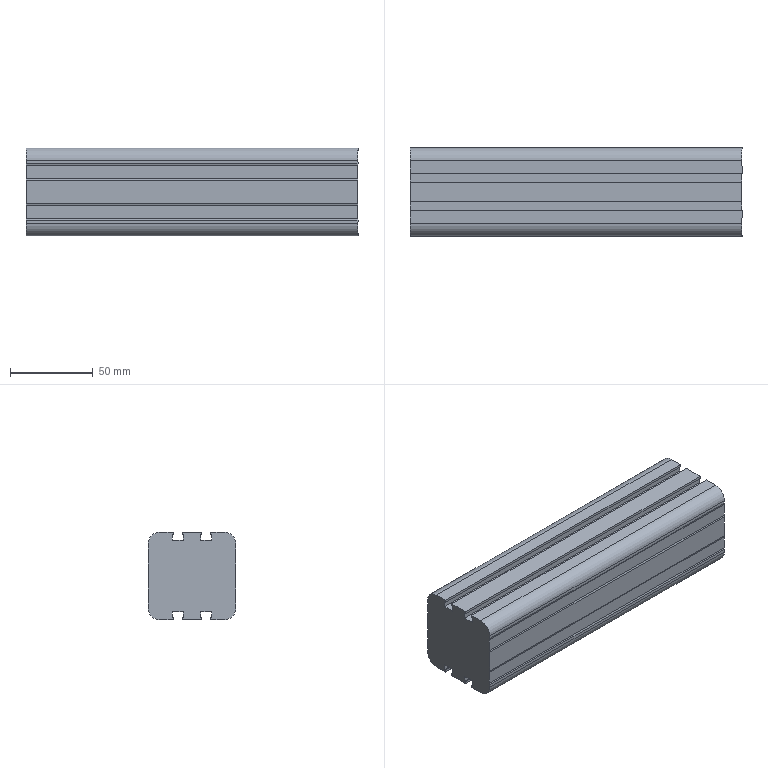Part | SolidWorks | features BaseBody 1 | 1 solid | 58 faces | box 200 x 53 x 53 mm | volume 525174 mm3 | plane 54 | cylinder 4 | commonest cylinder face diameters 15.1 x4